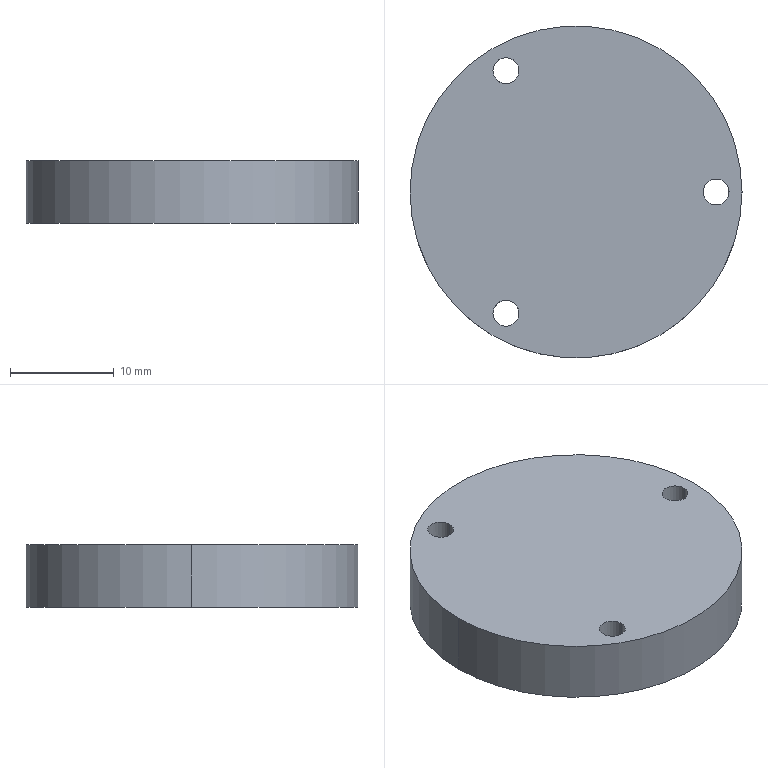Part | SolidWorks | features BaseBody 1 | 1 solid | 16 faces | box 32 x 32 x 6 mm | volume 4734 mm3 | cylinder 8 | spline 6 | plane 2 | commonest cylinder face diameters 2.5 x6 32 x2
STEP:
#1=CARTESIAN_POINT('',(14.75,0.,-0.3));
#2=VERTEX_POINT('',#1);
#3=CARTESIAN_POINT('',(12.25,0.,-0.3));
#4=VERTEX_POINT('',#3);
#5=CARTESIAN_POINT('',(13.5,0.,-0.3));
#6=DIRECTION('',(0.,0.,1.));
#7=DIRECTION('',(1.,0.,0.));
#8=AXIS2_PLACEMENT_3D('',#5,#6,#7);
#9=CIRCLE('',#8,1.25);
#10=EDGE_CURVE('',#2,#4,#9,.T.);
#11=ORIENTED_EDGE('',*,*,#10,.T.);
#12=CARTESIAN_POINT('',(11.55,0.,-1.));
#13=VERTEX_POINT('',#12);
#14=CARTESIAN_POINT('',(11.55,0.,-0.3));
#15=DIRECTION('',(0.,1.,0.));
#16=DIRECTION('',(-1.,0.,0.));
#17=AXIS2_PLACEMENT_3D('',#14,#15,#16);
#18=CIRCLE('',#17,0.7);
#19=EDGE_CURVE('',#4,#13,#18,.T.);
#20=ORIENTED_EDGE('',*,*,#19,.T.);
#21=CARTESIAN_POINT('',(15.45,0.,-1.));
#22=VERTEX_POINT('',#21);
#23=CARTESIAN_POINT('',(11.55,0.,-1.));
#24=CARTESIAN_POINT('',(11.55,3.9,-1.));
#25=CARTESIAN_POINT('',(15.45,3.9,-1.));
#26=CARTESIAN_POINT('',(15.45,0.,-1.));
#27=(BOUNDED_CURVE()B_SPLINE_CURVE(3,(#23,#24,#25,#26),.UNSPECIFIED.,.F.,.F.)B_SPLINE_CURVE_WITH_KNOTS((4,4),(0.5,1.),.UNSPECIFIED.)CURVE()GEOMETRIC_REPRESENTATION_ITEM()RATIONAL_B_SPLINE_CURVE((1.,0.3333,0.3333,1.))REPRESENTATION_ITEM(''));
#28=EDGE_CURVE('',#13,#22,#27,.T.);
#29=ORIENTED_EDGE('',*,*,#28,.T.);
#30=CARTESIAN_POINT('',(15.45,0.,-0.3));
#31=DIRECTION('',(0.,-1.,0.));
#32=DIRECTION('',(1.,0.,0.));
#33=AXIS2_PLACEMENT_3D('',#30,#31,#32);
#34=CIRCLE('',#33,0.7);
#35=EDGE_CURVE('',#2,#22,#34,.T.);
#36=ORIENTED_EDGE('',*,*,#35,.F.);
#37=EDGE_LOOP('',(#11,#20,#29,#36));
#38=FACE_OUTER_BOUND('',#37,.T.);
#39=CARTESIAN_POINT('',(12.25,0.,-0.3));
#40=CARTESIAN_POINT('',(12.25,2.5,-0.3));
#41=CARTESIAN_POINT('',(14.75,2.5,-0.3));
#42=CARTESIAN_POINT('',(14.75,0.,-0.3));
#43=CARTESIAN_POINT('',(12.25,0.,-0.7101));
#44=CARTESIAN_POINT('',(12.25,2.5,-0.7101));
#45=CARTESIAN_POINT('',(14.75,2.5,-0.7101));
#46=CARTESIAN_POINT('',(14.75,0.,-0.7101));
#47=CARTESIAN_POINT('',(11.96,0.,-1.));
#48=CARTESIAN_POINT('',(11.96,3.08,-1.));
#49=CARTESIAN_POINT('',(15.04,3.08,-1.));
#50=CARTESIAN_POINT('',(15.04,0.,-1.));
#51=CARTESIAN_POINT('',(11.55,0.,-1.));
#52=CARTESIAN_POINT('',(11.55,3.9,-1.));
#53=CARTESIAN_POINT('',(15.45,3.9,-1.));
#54=CARTESIAN_POINT('',(15.45,0.,-1.));
#55=(BOUNDED_SURFACE()B_SPLINE_SURFACE(3,3,((#39,#40,#41,#42),(#43,#44,#45,#46),(#47,#48,#49,#50),(#51,#52,#53,#54)),.UNSPECIFIED.,.F.,.F.,.T.)B_SPLINE_SURFACE_WITH_KNOTS((4,4),(4,4),(0.,1.),(0.,1.),.UNSPECIFIED.)GEOMETRIC_REPRESENTATION_ITEM()RATIONAL_B_SPLINE_SURFACE(((1.,0.3333,0.3333,1.),(0.8047,0.2682,0.2682,0.8047),(0.8047,0.2682,0.2682,0.8047),(1.,0.3333,0.3333,1.)))REPRESENTATION_ITEM('')SURFACE());
#56=ADVANCED_FACE('',(#38),#55,.T.);
#57=CARTESIAN_POINT('',(-8.,11.691,-0.3));
#58=VERTEX_POINT('',#57);
#59=CARTESIAN_POINT('',(-6.125,10.609,-0.3));
#60=VERTEX_POINT('',#59);
#61=CARTESIAN_POINT('',(-6.75,11.691,-0.3));
#62=DIRECTION('',(0.,0.,1.));
#63=DIRECTION('',(1.,0.,0.));
#64=AXIS2_PLACEMENT_3D('',#61,#62,#63);
#65=CIRCLE('',#64,1.25);
#66=EDGE_CURVE('',#58,#60,#65,.T.);
#67=ORIENTED_EDGE('',*,*,#66,.T.);
#68=CARTESIAN_POINT('',(-5.775,10.003,-1.));
#69=VERTEX_POINT('',#68);
#70=CARTESIAN_POINT('',(-5.775,10.003,-0.3));
#71=DIRECTION('',(-0.866,-0.5,0.));
#72=DIRECTION('',(0.5,-0.866,0.));
#73=AXIS2_PLACEMENT_3D('',#70,#71,#72);
#74=CIRCLE('',#73,0.7);
#75=EDGE_CURVE('',#60,#69,#74,.T.);
#76=ORIENTED_EDGE('',*,*,#75,.T.);
#77=CARTESIAN_POINT('',(-7.725,13.38,-1.));
#78=VERTEX_POINT('',#77);
#79=CARTESIAN_POINT('',(-5.775,10.003,-1.));
#80=CARTESIAN_POINT('',(-9.152,8.053,-1.));
#81=CARTESIAN_POINT('',(-11.102,11.43,-1.));
#82=CARTESIAN_POINT('',(-7.725,13.38,-1.));
#83=(BOUNDED_CURVE()B_SPLINE_CURVE(3,(#79,#80,#81,#82),.UNSPECIFIED.,.F.,.F.)B_SPLINE_CURVE_WITH_KNOTS((4,4),(0.5,1.),.UNSPECIFIED.)CURVE()GEOMETRIC_REPRESENTATION_ITEM()RATIONAL_B_SPLINE_CURVE((1.,0.3333,0.3333,1.))REPRESENTATION_ITEM(''));
#84=EDGE_CURVE('',#69,#78,#83,.T.);
#85=ORIENTED_EDGE('',*,*,#84,.T.);
#86=CARTESIAN_POINT('',(-7.375,12.774,-0.3));
#87=VERTEX_POINT('',#86);
#88=CARTESIAN_POINT('',(-7.725,13.38,-0.3));
#89=DIRECTION('',(0.866,0.5,0.));
#90=DIRECTION('',(-0.5,0.866,0.));
#91=AXIS2_PLACEMENT_3D('',#88,#89,#90);
#92=CIRCLE('',#91,0.7);
#93=EDGE_CURVE('',#87,#78,#92,.T.);
#94=ORIENTED_EDGE('',*,*,#93,.F.);
#95=CARTESIAN_POINT('',(-6.75,11.691,-0.3));
#96=DIRECTION('',(0.,0.,1.));
#97=DIRECTION('',(1.,0.,0.));
#98=AXIS2_PLACEMENT_3D('',#95,#96,#97);
#99=CIRCLE('',#98,1.25);
#100=EDGE_CURVE('',#87,#58,#99,.T.);
#101=ORIENTED_EDGE('',*,*,#100,.T.);
#102=EDGE_LOOP('',(#67,#76,#85,#94,#101));
#103=FACE_OUTER_BOUND('',#102,.T.);
#104=CARTESIAN_POINT('',(-6.125,10.609,-0.3));
#105=CARTESIAN_POINT('',(-8.29,9.359,-0.3));
#106=CARTESIAN_POINT('',(-9.54,11.524,-0.3));
#107=CARTESIAN_POINT('',(-7.375,12.774,-0.3));
#108=CARTESIAN_POINT('',(-6.125,10.609,-0.7101));
#109=CARTESIAN_POINT('',(-8.29,9.359,-0.7101));
#110=CARTESIAN_POINT('',(-9.54,11.524,-0.7101));
#111=CARTESIAN_POINT('',(-7.375,12.774,-0.7101));
#112=CARTESIAN_POINT('',(-5.98,10.358,-1.));
#113=CARTESIAN_POINT('',(-8.647,8.818,-1.));
#114=CARTESIAN_POINT('',(-10.187,11.485,-1.));
#115=CARTESIAN_POINT('',(-7.52,13.025,-1.));
#116=CARTESIAN_POINT('',(-5.775,10.003,-1.));
#117=CARTESIAN_POINT('',(-9.152,8.053,-1.));
#118=CARTESIAN_POINT('',(-11.102,11.43,-1.));
#119=CARTESIAN_POINT('',(-7.725,13.38,-1.));
#120=(BOUNDED_SURFACE()B_SPLINE_SURFACE(3,3,((#104,#105,#106,#107),(#108,#109,#110,#111),(#112,#113,#114,#115),(#116,#117,#118,#119)),.UNSPECIFIED.,.F.,.F.,.F.)B_SPLINE_SURFACE_WITH_KNOTS((4,4),(4,4),(0.,1.),(0.,1.),.UNSPECIFIED.)GEOMETRIC_REPRESENTATION_ITEM()RATIONAL_B_SPLINE_SURFACE(((1.,0.3333,0.3333,1.),(0.8047,0.2682,0.2682,0.8047),(0.8047,0.2682,0.2682,0.8047),(1.,0.3333,0.3333,1.)))REPRESENTATION_ITEM('')SURFACE());
#121=ADVANCED_FACE('',(#103),#120,.T.);
#122=CARTESIAN_POINT('',(-5.5,-11.691,-0.3));
#123=VERTEX_POINT('',#122);
#124=CARTESIAN_POINT('',(-6.125,-10.609,-0.3));
#125=VERTEX_POINT('',#124);
#126=CARTESIAN_POINT('',(-6.75,-11.691,-0.3));
#127=DIRECTION('',(0.,0.,1.));
#128=DIRECTION('',(1.,0.,0.));
#129=AXIS2_PLACEMENT_3D('',#126,#127,#128);
#130=CIRCLE('',#129,1.25);
#131=EDGE_CURVE('',#123,#125,#130,.T.);
#132=ORIENTED_EDGE('',*,*,#131,.T.);
#133=CARTESIAN_POINT('',(-5.775,-10.003,-1.));
#134=VERTEX_POINT('',#133);
#135=CARTESIAN_POINT('',(-5.775,-10.003,-0.3));
#136=DIRECTION('',(0.866,-0.5,0.));
#137=DIRECTION('',(0.5,0.866,0.));
#138=AXIS2_PLACEMENT_3D('',#135,#136,#137);
#139=CIRCLE('',#138,0.7);
#140=EDGE_CURVE('',#125,#134,#139,.T.);
#141=ORIENTED_EDGE('',*,*,#140,.T.);
#142=CARTESIAN_POINT('',(-7.725,-13.38,-1.));
#143=VERTEX_POINT('',#142);
#144=CARTESIAN_POINT('',(-5.775,-10.003,-1.));
#145=CARTESIAN_POINT('',(-2.398,-11.953,-1.));
#146=CARTESIAN_POINT('',(-4.348,-15.33,-1.));
#147=CARTESIAN_POINT('',(-7.725,-13.38,-1.));
#148=(BOUNDED_CURVE()B_SPLINE_CURVE(3,(#144,#145,#146,#147),.UNSPECIFIED.,.F.,.T.)B_SPLINE_CURVE_WITH_KNOTS((4,4),(0.5,1.),.UNSPECIFIED.)CURVE()GEOMETRIC_REPRESENTATION_ITEM()RATIONAL_B_SPLINE_CURVE((1.,0.3333,0.3333,1.))REPRESENTATION_ITEM(''));
#149=EDGE_CURVE('',#134,#143,#148,.T.);
#150=ORIENTED_EDGE('',*,*,#149,.T.);
#151=CARTESIAN_POINT('',(-7.375,-12.774,-0.3));
#152=VERTEX_POINT('',#151);
#153=CARTESIAN_POINT('',(-7.725,-13.38,-0.3));
#154=DIRECTION('',(-0.866,0.5,0.));
#155=DIRECTION('',(-0.5,-0.866,0.));
#156=AXIS2_PLACEMENT_3D('',#153,#154,#155);
#157=CIRCLE('',#156,0.7);
#158=EDGE_CURVE('',#152,#143,#157,.T.);
#159=ORIENTED_EDGE('',*,*,#158,.F.);
#160=CARTESIAN_POINT('',(-6.75,-11.691,-0.3));
#161=DIRECTION('',(0.,0.,1.));
#162=DIRECTION('',(1.,0.,0.));
#163=AXIS2_PLACEMENT_3D('',#160,#161,#162);
#164=CIRCLE('',#163,1.25);
#165=EDGE_CURVE('',#152,#123,#164,.T.);
#166=ORIENTED_EDGE('',*,*,#165,.T.);
#167=EDGE_LOOP('',(#132,#141,#150,#159,#166));
#168=FACE_OUTER_BOUND('',#167,.T.);
#169=CARTESIAN_POINT('',(-6.125,-10.609,-0.3));
#170=CARTESIAN_POINT('',(-3.96,-11.859,-0.3));
#171=CARTESIAN_POINT('',(-5.21,-14.024,-0.3));
#172=CARTESIAN_POINT('',(-7.375,-12.774,-0.3));
#173=CARTESIAN_POINT('',(-6.125,-10.609,-0.7101));
#174=CARTESIAN_POINT('',(-3.96,-11.859,-0.7101));
#175=CARTESIAN_POINT('',(-5.21,-14.024,-0.7101));
#176=CARTESIAN_POINT('',(-7.375,-12.774,-0.7101));
#177=CARTESIAN_POINT('',(-5.98,-10.358,-1.));
#178=CARTESIAN_POINT('',(-3.313,-11.898,-1.));
#179=CARTESIAN_POINT('',(-4.853,-14.565,-1.));
#180=CARTESIAN_POINT('',(-7.52,-13.025,-1.));
#181=CARTESIAN_POINT('',(-5.775,-10.003,-1.));
#182=CARTESIAN_POINT('',(-2.398,-11.953,-1.));
#183=CARTESIAN_POINT('',(-4.348,-15.33,-1.));
#184=CARTESIAN_POINT('',(-7.725,-13.38,-1.));
#185=(BOUNDED_SURFACE()B_SPLINE_SURFACE(3,3,((#169,#170,#171,#172),(#173,#174,#175,#176),(#177,#178,#179,#180),(#181,#182,#183,#184)),.UNSPECIFIED.,.F.,.F.,.T.)B_SPLINE_SURFACE_WITH_KNOTS((4,4),(4,4),(0.,1.),(0.,1.),.UNSPECIFIED.)GEOMETRIC_REPRESENTATION_ITEM()RATIONAL_B_SPLINE_SURFACE(((1.,0.3333,0.3333,1.),(0.8047,0.2682,0.2682,0.8047),(0.8047,0.2682,0.2682,0.8047),(1.,0.3333,0.3333,1.)))REPRESENTATION_ITEM('')SURFACE());
#186=ADVANCED_FACE('',(#168),#185,.T.);
#187=CARTESIAN_POINT('',(13.5,0.,-0.3));
#188=DIRECTION('',(0.,0.,1.));
#189=DIRECTION('',(1.,0.,0.));
#190=AXIS2_PLACEMENT_3D('',#187,#188,#189);
#191=CIRCLE('',#190,1.25);
#192=EDGE_CURVE('',#4,#2,#191,.T.);
#193=ORIENTED_EDGE('',*,*,#192,.F.);
#194=CARTESIAN_POINT('',(12.25,0.,5.));
#195=VERTEX_POINT('',#194);
#196=CARTESIAN_POINT('',(12.25,0.,5.));
#197=DIRECTION('',(0.,0.,1.));
#198=VECTOR('',#197,1000.);
#199=LINE('',#196,#198);
#200=EDGE_CURVE('',#4,#195,#199,.T.);
#201=ORIENTED_EDGE('',*,*,#200,.T.);
#202=CARTESIAN_POINT('',(14.75,0.,5.));
#203=VERTEX_POINT('',#202);
#204=CARTESIAN_POINT('',(13.5,0.,5.));
#205=DIRECTION('',(0.,0.,-1.));
#206=DIRECTION('',(1.,0.,0.));
#207=AXIS2_PLACEMENT_3D('',#204,#205,#206);
#208=CIRCLE('',#207,1.25);
#209=EDGE_CURVE('',#203,#195,#208,.T.);
#210=ORIENTED_EDGE('',*,*,#209,.F.);
#211=CARTESIAN_POINT('',(14.75,0.,5.));
#212=DIRECTION('',(0.,0.,1.));
#213=VECTOR('',#212,1000.);
#214=LINE('',#211,#213);
#215=EDGE_CURVE('',#2,#203,#214,.T.);
#216=ORIENTED_EDGE('',*,*,#215,.F.);
#217=EDGE_LOOP('',(#193,#201,#210,#216));
#218=FACE_OUTER_BOUND('',#217,.T.);
#219=CARTESIAN_POINT('',(13.5,0.,5.));
#220=DIRECTION('',(0.,0.,1.));
#221=DIRECTION('',(1.,0.,0.));
#222=AXIS2_PLACEMENT_3D('',#219,#220,#221);
#223=CYLINDRICAL_SURFACE('',#222,1.25);
#224=ADVANCED_FACE('',(#218),#223,.F.);
#225=ORIENTED_EDGE('',*,*,#66,.F.);
#226=CARTESIAN_POINT('',(-8.,11.691,5.));
#227=VERTEX_POINT('',#226);
#228=CARTESIAN_POINT('',(-8.,11.691,5.));
#229=DIRECTION('',(0.,0.,1.));
#230=VECTOR('',#229,1000.);
#231=LINE('',#228,#230);
#232=EDGE_CURVE('',#58,#227,#231,.T.);
#233=ORIENTED_EDGE('',*,*,#232,.T.);
#234=CARTESIAN_POINT('',(-5.5,11.691,5.));
#235=VERTEX_POINT('',#234);
#236=CARTESIAN_POINT('',(-6.75,11.691,5.));
#237=DIRECTION('',(0.,0.,-1.));
#238=DIRECTION('',(1.,0.,0.));
#239=AXIS2_PLACEMENT_3D('',#236,#237,#238);
#240=CIRCLE('',#239,1.25);
#241=EDGE_CURVE('',#235,#227,#240,.T.);
#242=ORIENTED_EDGE('',*,*,#241,.F.);
#243=CARTESIAN_POINT('',(-5.5,11.691,-0.3));
#244=VERTEX_POINT('',#243);
#245=CARTESIAN_POINT('',(-5.5,11.691,5.));
#246=DIRECTION('',(0.,0.,1.));
#247=VECTOR('',#246,1000.);
#248=LINE('',#245,#247);
#249=EDGE_CURVE('',#244,#235,#248,.T.);
#250=ORIENTED_EDGE('',*,*,#249,.F.);
#251=CARTESIAN_POINT('',(-6.75,11.691,-0.3));
#252=DIRECTION('',(0.,0.,1.));
#253=DIRECTION('',(1.,0.,0.));
#254=AXIS2_PLACEMENT_3D('',#251,#252,#253);
#255=CIRCLE('',#254,1.25);
#256=EDGE_CURVE('',#60,#244,#255,.T.);
#257=ORIENTED_EDGE('',*,*,#256,.F.);
#258=EDGE_LOOP('',(#225,#233,#242,#250,#257));
#259=FACE_OUTER_BOUND('',#258,.T.);
#260=CARTESIAN_POINT('',(-6.75,11.691,5.));
#261=DIRECTION('',(0.,0.,1.));
#262=DIRECTION('',(1.,0.,0.));
#263=AXIS2_PLACEMENT_3D('',#260,#261,#262);
#264=CYLINDRICAL_SURFACE('',#263,1.25);
#265=ADVANCED_FACE('',(#259),#264,.F.);
#266=CARTESIAN_POINT('',(-8.,-11.691,-0.3));
#267=VERTEX_POINT('',#266);
#268=CARTESIAN_POINT('',(-6.75,-11.691,-0.3));
#269=DIRECTION('',(0.,0.,1.));
#270=DIRECTION('',(1.,0.,0.));
#271=AXIS2_PLACEMENT_3D('',#268,#269,#270);
#272=CIRCLE('',#271,1.25);
#273=EDGE_CURVE('',#267,#152,#272,.T.);
#274=ORIENTED_EDGE('',*,*,#273,.F.);
#275=CARTESIAN_POINT('',(-8.,-11.691,5.));
#276=VERTEX_POINT('',#275);
#277=CARTESIAN_POINT('',(-8.,-11.691,5.));
#278=DIRECTION('',(0.,0.,1.));
#279=VECTOR('',#278,1000.);
#280=LINE('',#277,#279);
#281=EDGE_CURVE('',#267,#276,#280,.T.);
#282=ORIENTED_EDGE('',*,*,#281,.T.);
#283=CARTESIAN_POINT('',(-5.5,-11.691,5.));
#284=VERTEX_POINT('',#283);
#285=CARTESIAN_POINT('',(-6.75,-11.691,5.));
#286=DIRECTION('',(0.,0.,-1.));
#287=DIRECTION('',(1.,0.,0.));
#288=AXIS2_PLACEMENT_3D('',#285,#286,#287);
#289=CIRCLE('',#288,1.25);
#290=EDGE_CURVE('',#284,#276,#289,.T.);
#291=ORIENTED_EDGE('',*,*,#290,.F.);
#292=CARTESIAN_POINT('',(-5.5,-11.691,5.));
#293=DIRECTION('',(0.,0.,1.));
#294=VECTOR('',#293,1000.);
#295=LINE('',#292,#294);
#296=EDGE_CURVE('',#123,#284,#295,.T.);
#297=ORIENTED_EDGE('',*,*,#296,.F.);
#298=ORIENTED_EDGE('',*,*,#165,.F.);
#299=EDGE_LOOP('',(#274,#282,#291,#297,#298));
#300=FACE_OUTER_BOUND('',#299,.T.);
#301=CARTESIAN_POINT('',(-6.75,-11.691,5.));
#302=DIRECTION('',(0.,0.,1.));
#303=DIRECTION('',(1.,0.,0.));
#304=AXIS2_PLACEMENT_3D('',#301,#302,#303);
#305=CYLINDRICAL_SURFACE('',#304,1.25);
#306=ADVANCED_FACE('',(#300),#305,.F.);
#307=CARTESIAN_POINT('',(16.,0.,-1.));
#308=VERTEX_POINT('',#307);
#309=CARTESIAN_POINT('',(-16.,0.,-1.));
#310=VERTEX_POINT('',#309);
#311=CARTESIAN_POINT('',(0.,0.,-1.));
#312=DIRECTION('',(0.,0.,1.));
#313=DIRECTION('',(1.,0.,0.));
#314=AXIS2_PLACEMENT_3D('',#311,#312,#313);
#315=CIRCLE('',#314,16.);
#316=EDGE_CURVE('',#308,#310,#315,.T.);
#317=ORIENTED_EDGE('',*,*,#316,.T.);
#318=CARTESIAN_POINT('',(-16.,0.,5.));
#319=VERTEX_POINT('',#318);
#320=CARTESIAN_POINT('',(-16.,0.,-1.));
#321=DIRECTION('',(0.,0.,1.));
#322=VECTOR('',#321,1000.);
#323=LINE('',#320,#322);
#324=EDGE_CURVE('',#310,#319,#323,.T.);
#325=ORIENTED_EDGE('',*,*,#324,.T.);
#326=CARTESIAN_POINT('',(16.,0.,5.));
#327=VERTEX_POINT('',#326);
#328=CARTESIAN_POINT('',(0.,0.,5.));
#329=DIRECTION('',(0.,0.,1.));
#330=DIRECTION('',(1.,0.,0.));
#331=AXIS2_PLACEMENT_3D('',#328,#329,#330);
#332=CIRCLE('',#331,16.);
#333=EDGE_CURVE('',#327,#319,#332,.T.);
#334=ORIENTED_EDGE('',*,*,#333,.F.);
#335=CARTESIAN_POINT('',(16.,0.,-1.));
#336=DIRECTION('',(0.,0.,1.));
#337=VECTOR('',#336,1000.);
#338=LINE('',#335,#337);
#339=EDGE_CURVE('',#308,#327,#338,.T.);
#340=ORIENTED_EDGE('',*,*,#339,.F.);
#341=EDGE_LOOP('',(#317,#325,#334,#340));
#342=FACE_OUTER_BOUND('',#341,.T.);
#343=CARTESIAN_POINT('',(0.,0.,-1.));
#344=DIRECTION('',(0.,0.,1.));
#345=DIRECTION('',(1.,0.,0.));
#346=AXIS2_PLACEMENT_3D('',#343,#344,#345);
#347=CYLINDRICAL_SURFACE('',#346,16.);
#348=ADVANCED_FACE('',(#342),#347,.T.);
#349=ORIENTED_EDGE('',*,*,#209,.T.);
#350=CARTESIAN_POINT('',(13.5,0.,5.));
#351=DIRECTION('',(0.,0.,-1.));
#352=DIRECTION('',(1.,0.,0.));
#353=AXIS2_PLACEMENT_3D('',#350,#351,#352);
#354=CIRCLE('',#353,1.25);
#355=EDGE_CURVE('',#195,#203,#354,.T.);
#356=ORIENTED_EDGE('',*,*,#355,.T.);
#357=EDGE_LOOP('',(#349,#356));
#358=FACE_BOUND('',#357,.T.);
#359=ORIENTED_EDGE('',*,*,#241,.T.);
#360=CARTESIAN_POINT('',(-6.75,11.691,5.));
#361=DIRECTION('',(0.,0.,-1.));
#362=DIRECTION('',(1.,0.,0.));
#363=AXIS2_PLACEMENT_3D('',#360,#361,#362);
#364=CIRCLE('',#363,1.25);
#365=EDGE_CURVE('',#227,#235,#364,.T.);
#366=ORIENTED_EDGE('',*,*,#365,.T.);
#367=EDGE_LOOP('',(#359,#366));
#368=FACE_BOUND('',#367,.T.);
#369=ORIENTED_EDGE('',*,*,#290,.T.);
#370=CARTESIAN_POINT('',(-6.75,-11.691,5.));
#371=DIRECTION('',(0.,0.,-1.));
#372=DIRECTION('',(1.,0.,0.));
#373=AXIS2_PLACEMENT_3D('',#370,#371,#372);
#374=CIRCLE('',#373,1.25);
#375=EDGE_CURVE('',#276,#284,#374,.T.);
#376=ORIENTED_EDGE('',*,*,#375,.T.);
#377=EDGE_LOOP('',(#369,#376));
#378=FACE_BOUND('',#377,.T.);
#379=ORIENTED_EDGE('',*,*,#333,.T.);
#380=CARTESIAN_POINT('',(0.,0.,5.));
#381=DIRECTION('',(0.,0.,1.));
#382=DIRECTION('',(1.,0.,0.));
#383=AXIS2_PLACEMENT_3D('',#380,#381,#382);
#384=CIRCLE('',#383,16.);
#385=EDGE_CURVE('',#319,#327,#384,.T.);
#386=ORIENTED_EDGE('',*,*,#385,.T.);
#387=EDGE_LOOP('',(#379,#386));
#388=FACE_OUTER_BOUND('',#387,.T.);
#389=CARTESIAN_POINT('',(0.,0.,5.));
#390=DIRECTION('',(0.,0.,1.));
#391=DIRECTION('',(1.,0.,0.));
#392=AXIS2_PLACEMENT_3D('',#389,#390,#391);
#393=PLANE('',#392);
#394=ADVANCED_FACE('',(#358,#368,#378,#388),#393,.T.);
#395=ORIENTED_EDGE('',*,*,#200,.F.);
#396=ORIENTED_EDGE('',*,*,#10,.F.);
#397=ORIENTED_EDGE('',*,*,#215,.T.);
#398=ORIENTED_EDGE('',*,*,#355,.F.);
#399=EDGE_LOOP('',(#395,#396,#397,#398));
#400=FACE_OUTER_BOUND('',#399,.T.);
#401=CARTESIAN_POINT('',(13.5,0.,5.));
#402=DIRECTION('',(0.,0.,1.));
#403=DIRECTION('',(1.,0.,0.));
#404=AXIS2_PLACEMENT_3D('',#401,#402,#403);
#405=CYLINDRICAL_SURFACE('',#404,1.25);
#406=ADVANCED_FACE('',(#400),#405,.F.);
#407=ORIENTED_EDGE('',*,*,#232,.F.);
#408=ORIENTED_EDGE('',*,*,#100,.F.);
#409=CARTESIAN_POINT('',(-6.75,11.691,-0.3));
#410=DIRECTION('',(0.,0.,1.));
#411=DIRECTION('',(1.,0.,0.));
#412=AXIS2_PLACEMENT_3D('',#409,#410,#411);
#413=CIRCLE('',#412,1.25);
#414=EDGE_CURVE('',#244,#87,#413,.T.);
#415=ORIENTED_EDGE('',*,*,#414,.F.);
#416=ORIENTED_EDGE('',*,*,#249,.T.);
#417=ORIENTED_EDGE('',*,*,#365,.F.);
#418=EDGE_LOOP('',(#407,#408,#415,#416,#417));
#419=FACE_OUTER_BOUND('',#418,.T.);
#420=CARTESIAN_POINT('',(-6.75,11.691,5.));
#421=DIRECTION('',(0.,0.,1.));
#422=DIRECTION('',(1.,0.,0.));
#423=AXIS2_PLACEMENT_3D('',#420,#421,#422);
#424=CYLINDRICAL_SURFACE('',#423,1.25);
#425=ADVANCED_FACE('',(#419),#424,.F.);
#426=ORIENTED_EDGE('',*,*,#281,.F.);
#427=CARTESIAN_POINT('',(-6.75,-11.691,-0.3));
#428=DIRECTION('',(0.,0.,1.));
#429=DIRECTION('',(1.,0.,0.));
#430=AXIS2_PLACEMENT_3D('',#427,#428,#429);
#431=CIRCLE('',#430,1.25);
#432=EDGE_CURVE('',#125,#267,#431,.T.);
#433=ORIENTED_EDGE('',*,*,#432,.F.);
#434=ORIENTED_EDGE('',*,*,#131,.F.);
#435=ORIENTED_EDGE('',*,*,#296,.T.);
#436=ORIENTED_EDGE('',*,*,#375,.F.);
#437=EDGE_LOOP('',(#426,#433,#434,#435,#436));
#438=FACE_OUTER_BOUND('',#437,.T.);
#439=CARTESIAN_POINT('',(-6.75,-11.691,5.));
#440=DIRECTION('',(0.,0.,1.));
#441=DIRECTION('',(1.,0.,0.));
#442=AXIS2_PLACEMENT_3D('',#439,#440,#441);
#443=CYLINDRICAL_SURFACE('',#442,1.25);
#444=ADVANCED_FACE('',(#438),#443,.F.);
#445=ORIENTED_EDGE('',*,*,#324,.F.);
#446=CARTESIAN_POINT('',(0.,0.,-1.));
#447=DIRECTION('',(0.,0.,1.));
#448=DIRECTION('',(1.,0.,0.));
#449=AXIS2_PLACEMENT_3D('',#446,#447,#448);
#450=CIRCLE('',#449,16.);
#451=EDGE_CURVE('',#310,#308,#450,.T.);
#452=ORIENTED_EDGE('',*,*,#451,.T.);
#453=ORIENTED_EDGE('',*,*,#339,.T.);
#454=ORIENTED_EDGE('',*,*,#385,.F.);
#455=EDGE_LOOP('',(#445,#452,#453,#454));
#456=FACE_OUTER_BOUND('',#455,.T.);
#457=CARTESIAN_POINT('',(0.,0.,-1.));
#458=DIRECTION('',(0.,0.,1.));
#459=DIRECTION('',(1.,0.,0.));
#460=AXIS2_PLACEMENT_3D('',#457,#458,#459);
#461=CYLINDRICAL_SURFACE('',#460,16.);
#462=ADVANCED_FACE('',(#456),#461,.T.);
#463=ORIENTED_EDGE('',*,*,#19,.F.);
#464=ORIENTED_EDGE('',*,*,#192,.T.);
#465=ORIENTED_EDGE('',*,*,#35,.T.);
#466=CARTESIAN_POINT('',(15.45,0.,-1.));
#467=CARTESIAN_POINT('',(15.45,-3.9,-1.));
#468=CARTESIAN_POINT('',(11.55,-3.9,-1.));
#469=CARTESIAN_POINT('',(11.55,0.,-1.));
#470=(BOUNDED_CURVE()B_SPLINE_CURVE(3,(#466,#467,#468,#469),.UNSPECIFIED.,.F.,.T.)B_SPLINE_CURVE_WITH_KNOTS((4,4),(0.,0.5),.UNSPECIFIED.)CURVE()GEOMETRIC_REPRESENTATION_ITEM()RATIONAL_B_SPLINE_CURVE((1.,0.3333,0.3333,1.))REPRESENTATION_ITEM(''));
#471=EDGE_CURVE('',#22,#13,#470,.T.);
#472=ORIENTED_EDGE('',*,*,#471,.T.);
#473=EDGE_LOOP('',(#463,#464,#465,#472));
#474=FACE_OUTER_BOUND('',#473,.T.);
#475=CARTESIAN_POINT('',(14.75,0.,-0.3));
#476=CARTESIAN_POINT('',(14.75,-2.5,-0.3));
#477=CARTESIAN_POINT('',(12.25,-2.5,-0.3));
#478=CARTESIAN_POINT('',(12.25,0.,-0.3));
#479=CARTESIAN_POINT('',(14.75,0.,-0.7101));
#480=CARTESIAN_POINT('',(14.75,-2.5,-0.7101));
#481=CARTESIAN_POINT('',(12.25,-2.5,-0.7101));
#482=CARTESIAN_POINT('',(12.25,0.,-0.7101));
#483=CARTESIAN_POINT('',(15.04,0.,-1.));
#484=CARTESIAN_POINT('',(15.04,-3.08,-1.));
#485=CARTESIAN_POINT('',(11.96,-3.08,-1.));
#486=CARTESIAN_POINT('',(11.96,0.,-1.));
#487=CARTESIAN_POINT('',(15.45,0.,-1.));
#488=CARTESIAN_POINT('',(15.45,-3.9,-1.));
#489=CARTESIAN_POINT('',(11.55,-3.9,-1.));
#490=CARTESIAN_POINT('',(11.55,0.,-1.));
#491=(BOUNDED_SURFACE()B_SPLINE_SURFACE(3,3,((#475,#476,#477,#478),(#479,#480,#481,#482),(#483,#484,#485,#486),(#487,#488,#489,#490)),.UNSPECIFIED.,.F.,.F.,.T.)B_SPLINE_SURFACE_WITH_KNOTS((4,4),(4,4),(0.,1.),(0.,1.),.UNSPECIFIED.)GEOMETRIC_REPRESENTATION_ITEM()RATIONAL_B_SPLINE_SURFACE(((1.,0.3333,0.3333,1.),(0.8047,0.2682,0.2682,0.8047),(0.8047,0.2682,0.2682,0.8047),(1.,0.3333,0.3333,1.)))REPRESENTATION_ITEM('')SURFACE());
#492=ADVANCED_FACE('',(#474),#491,.T.);
#493=ORIENTED_EDGE('',*,*,#75,.F.);
#494=ORIENTED_EDGE('',*,*,#256,.T.);
#495=ORIENTED_EDGE('',*,*,#414,.T.);
#496=ORIENTED_EDGE('',*,*,#93,.T.);
#497=CARTESIAN_POINT('',(-7.725,13.38,-1.));
#498=CARTESIAN_POINT('',(-4.348,15.33,-1.));
#499=CARTESIAN_POINT('',(-2.398,11.953,-1.));
#500=CARTESIAN_POINT('',(-5.775,10.003,-1.));
#501=(BOUNDED_CURVE()B_SPLINE_CURVE(3,(#497,#498,#499,#500),.UNSPECIFIED.,.F.,.T.)B_SPLINE_CURVE_WITH_KNOTS((4,4),(0.,0.5),.UNSPECIFIED.)CURVE()GEOMETRIC_REPRESENTATION_ITEM()RATIONAL_B_SPLINE_CURVE((1.,0.3333,0.3333,1.))REPRESENTATION_ITEM(''));
#502=EDGE_CURVE('',#78,#69,#501,.T.);
#503=ORIENTED_EDGE('',*,*,#502,.T.);
#504=EDGE_LOOP('',(#493,#494,#495,#496,#503));
#505=FACE_OUTER_BOUND('',#504,.T.);
#506=CARTESIAN_POINT('',(-7.375,12.774,-0.3));
#507=CARTESIAN_POINT('',(-5.21,14.024,-0.3));
#508=CARTESIAN_POINT('',(-3.96,11.859,-0.3));
#509=CARTESIAN_POINT('',(-6.125,10.609,-0.3));
#510=CARTESIAN_POINT('',(-7.375,12.774,-0.7101));
#511=CARTESIAN_POINT('',(-5.21,14.024,-0.7101));
#512=CARTESIAN_POINT('',(-3.96,11.859,-0.7101));
#513=CARTESIAN_POINT('',(-6.125,10.609,-0.7101));
#514=CARTESIAN_POINT('',(-7.52,13.025,-1.));
#515=CARTESIAN_POINT('',(-4.853,14.565,-1.));
#516=CARTESIAN_POINT('',(-3.313,11.898,-1.));
#517=CARTESIAN_POINT('',(-5.98,10.358,-1.));
#518=CARTESIAN_POINT('',(-7.725,13.38,-1.));
#519=CARTESIAN_POINT('',(-4.348,15.33,-1.));
#520=CARTESIAN_POINT('',(-2.398,11.953,-1.));
#521=CARTESIAN_POINT('',(-5.775,10.003,-1.));
#522=(BOUNDED_SURFACE()B_SPLINE_SURFACE(3,3,((#506,#507,#508,#509),(#510,#511,#512,#513),(#514,#515,#516,#517),(#518,#519,#520,#521)),.UNSPECIFIED.,.F.,.F.,.T.)B_SPLINE_SURFACE_WITH_KNOTS((4,4),(4,4),(0.,1.),(0.,1.),.UNSPECIFIED.)GEOMETRIC_REPRESENTATION_ITEM()RATIONAL_B_SPLINE_SURFACE(((1.,0.3333,0.3333,1.),(0.8047,0.2682,0.2682,0.8047),(0.8047,0.2682,0.2682,0.8047),(1.,0.3333,0.3333,1.)))REPRESENTATION_ITEM('')SURFACE());
#523=ADVANCED_FACE('',(#505),#522,.T.);
#524=ORIENTED_EDGE('',*,*,#140,.F.);
#525=ORIENTED_EDGE('',*,*,#432,.T.);
#526=ORIENTED_EDGE('',*,*,#273,.T.);
#527=ORIENTED_EDGE('',*,*,#158,.T.);
#528=CARTESIAN_POINT('',(-7.725,-13.38,-1.));
#529=CARTESIAN_POINT('',(-11.102,-11.43,-1.));
#530=CARTESIAN_POINT('',(-9.152,-8.053,-1.));
#531=CARTESIAN_POINT('',(-5.775,-10.003,-1.));
#532=(BOUNDED_CURVE()B_SPLINE_CURVE(3,(#528,#529,#530,#531),.UNSPECIFIED.,.F.,.F.)B_SPLINE_CURVE_WITH_KNOTS((4,4),(0.,0.5),.UNSPECIFIED.)CURVE()GEOMETRIC_REPRESENTATION_ITEM()RATIONAL_B_SPLINE_CURVE((1.,0.3333,0.3333,1.))REPRESENTATION_ITEM(''));
#533=EDGE_CURVE('',#143,#134,#532,.T.);
#534=ORIENTED_EDGE('',*,*,#533,.T.);
#535=EDGE_LOOP('',(#524,#525,#526,#527,#534));
#536=FACE_OUTER_BOUND('',#535,.T.);
#537=CARTESIAN_POINT('',(-7.375,-12.774,-0.3));
#538=CARTESIAN_POINT('',(-9.54,-11.524,-0.3));
#539=CARTESIAN_POINT('',(-8.29,-9.359,-0.3));
#540=CARTESIAN_POINT('',(-6.125,-10.609,-0.3));
#541=CARTESIAN_POINT('',(-7.375,-12.774,-0.7101));
#542=CARTESIAN_POINT('',(-9.54,-11.524,-0.7101));
#543=CARTESIAN_POINT('',(-8.29,-9.359,-0.7101));
#544=CARTESIAN_POINT('',(-6.125,-10.609,-0.7101));
#545=CARTESIAN_POINT('',(-7.52,-13.025,-1.));
#546=CARTESIAN_POINT('',(-10.187,-11.485,-1.));
#547=CARTESIAN_POINT('',(-8.647,-8.818,-1.));
#548=CARTESIAN_POINT('',(-5.98,-10.358,-1.));
#549=CARTESIAN_POINT('',(-7.725,-13.38,-1.));
#550=CARTESIAN_POINT('',(-11.102,-11.43,-1.));
#551=CARTESIAN_POINT('',(-9.152,-8.053,-1.));
#552=CARTESIAN_POINT('',(-5.775,-10.003,-1.));
#553=(BOUNDED_SURFACE()B_SPLINE_SURFACE(3,3,((#537,#538,#539,#540),(#541,#542,#543,#544),(#545,#546,#547,#548),(#549,#550,#551,#552)),.UNSPECIFIED.,.F.,.F.,.T.)B_SPLINE_SURFACE_WITH_KNOTS((4,4),(4,4),(0.,1.),(0.,1.),.UNSPECIFIED.)GEOMETRIC_REPRESENTATION_ITEM()RATIONAL_B_SPLINE_SURFACE(((1.,0.3333,0.3333,1.),(0.8047,0.2682,0.2682,0.8047),(0.8047,0.2682,0.2682,0.8047),(1.,0.3333,0.3333,1.)))REPRESENTATION_ITEM('')SURFACE());
#554=ADVANCED_FACE('',(#536),#553,.T.);
#555=ORIENTED_EDGE('',*,*,#533,.F.);
#556=ORIENTED_EDGE('',*,*,#149,.F.);
#557=EDGE_LOOP('',(#555,#556));
#558=FACE_BOUND('',#557,.T.);
#559=ORIENTED_EDGE('',*,*,#471,.F.);
#560=ORIENTED_EDGE('',*,*,#28,.F.);
#561=EDGE_LOOP('',(#559,#560));
#562=FACE_BOUND('',#561,.T.);
#563=ORIENTED_EDGE('',*,*,#316,.F.);
#564=ORIENTED_EDGE('',*,*,#451,.F.);
#565=EDGE_LOOP('',(#563,#564));
#566=FACE_OUTER_BOUND('',#565,.T.);
#567=ORIENTED_EDGE('',*,*,#502,.F.);
#568=ORIENTED_EDGE('',*,*,#84,.F.);
#569=EDGE_LOOP('',(#567,#568));
#570=FACE_BOUND('',#569,.T.);
#571=CARTESIAN_POINT('',(0.,0.,-1.));
#572=DIRECTION('',(0.,0.,1.));
#573=DIRECTION('',(1.,0.,0.));
#574=AXIS2_PLACEMENT_3D('',#571,#572,#573);
#575=PLANE('',#574);
#576=ADVANCED_FACE('',(#558,#562,#566,#570),#575,.F.);
#577=CLOSED_SHELL('',(#56,#121,#186,#224,#265,#306,#348,#394,#406,#425,#444,#462,#492,#523,#554,#576));
#578=MANIFOLD_SOLID_BREP('',#577);
#579=CARTESIAN_POINT('',(0.,0.,0.));
#580=DIRECTION('',(0.,0.,1.));
#581=DIRECTION('',(1.,0.,0.));
#582=AXIS2_PLACEMENT_3D('',#579,#580,#581);
#583=(LENGTH_UNIT()NAMED_UNIT(*)SI_UNIT(.MILLI.,.METRE.));
#584=UNCERTAINTY_MEASURE_WITH_UNIT(LENGTH_MEASURE(0.00001),#583,'','');
#585=(NAMED_UNIT(*)PLANE_ANGLE_UNIT()SI_UNIT($,.RADIAN.));
#586=(NAMED_UNIT(*)SI_UNIT($,.STERADIAN.)SOLID_ANGLE_UNIT());
#587=(GEOMETRIC_REPRESENTATION_CONTEXT(3)GLOBAL_UNCERTAINTY_ASSIGNED_CONTEXT((#584))GLOBAL_UNIT_ASSIGNED_CONTEXT((#583,#585,#586))REPRESENTATION_CONTEXT('',''));
#588=ADVANCED_BREP_SHAPE_REPRESENTATION('',(#578,#582),#587);